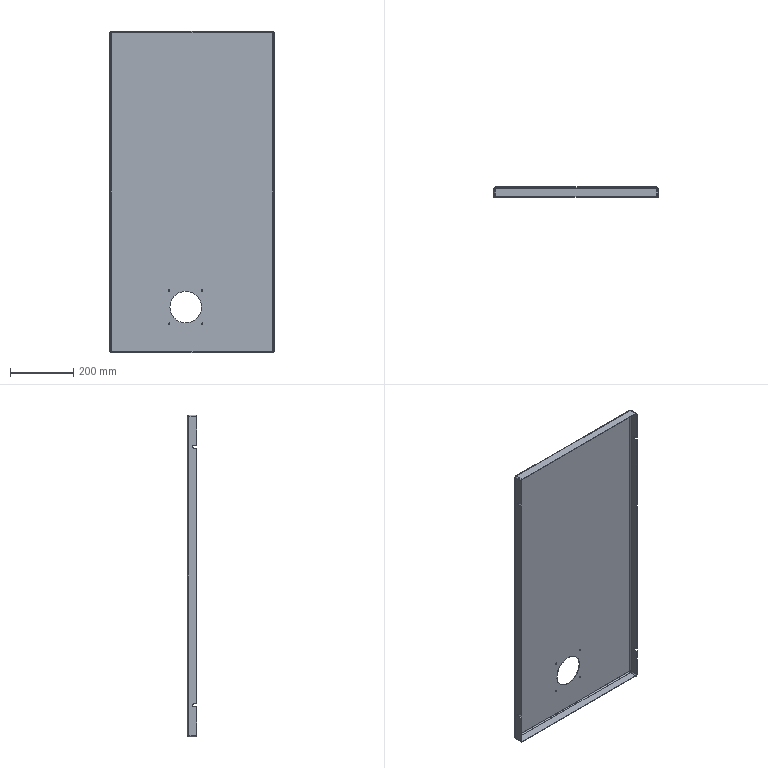Part | STEP file | 1 solid | 60 faces | box 520 x 30 x 1020 mm | volume 905709 mm3 | cylinder 30 | plane 22 | spline 8 | commonest cylinder face diameters 4.5 x8 7 x8 10 x8 8.5 x4 100 x2